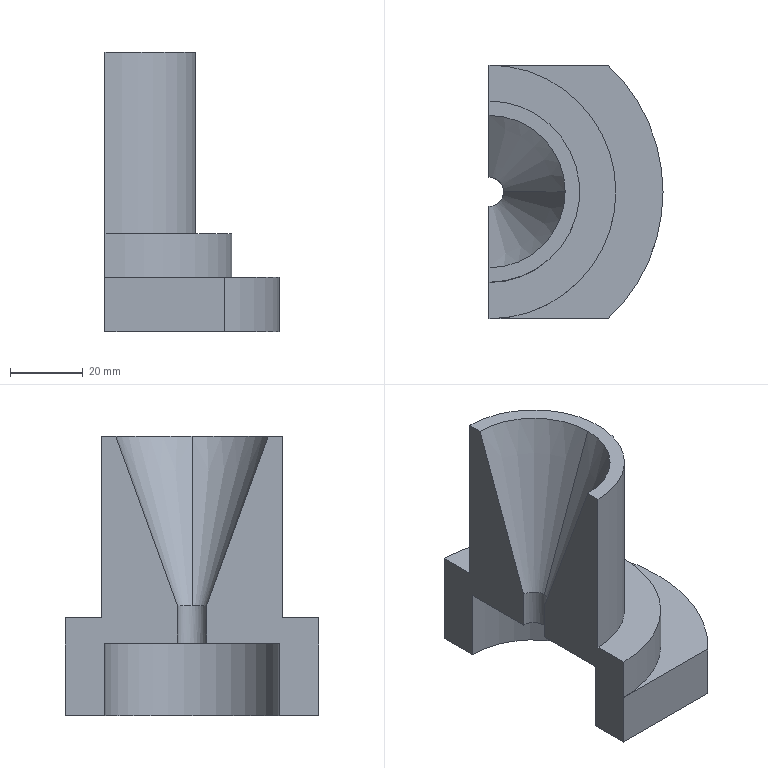Part | STEP file | 001-005-Shaft threading fixture mould | 1 solid | 16 faces | box 48 x 70 x 77 mm | volume 85963 mm3 | plane 9 | cylinder 5 | cone 2 | commonest cylinder face diameters 8.04 x1 48.1 x1 50 x1 70 x1 96 x1
STEP:
#1=CARTESIAN_POINT('',(0.,0.,0.));
#2=DIRECTION('',(0.,0.,1.));
#3=DIRECTION('',(1.,0.,0.));
#4=AXIS2_PLACEMENT_3D('',#1,#2,#3);
#5=CARTESIAN_POINT('',(0.,4.02,30.293));
#6=VERTEX_POINT('',#5);
#7=CARTESIAN_POINT('',(0.,21.02,77.));
#8=VERTEX_POINT('',#7);
#9=CARTESIAN_POINT('',(0.,0.,19.248));
#10=DIRECTION('',(0.,0.342,0.9397));
#11=VECTOR('',#10,1.);
#12=LINE('',#9,#11);
#13=CARTESIAN_POINT('',(0.,0.,77.));
#14=DIRECTION('',(0.,0.,1.));
#15=DIRECTION('',(1.,0.,0.));
#16=AXIS2_PLACEMENT_3D('',#13,#14,#15);
#17=CONICAL_SURFACE('',#16,21.02,0.3491);
#18=CARTESIAN_POINT('',(1.571,-57.752));
#19=DIRECTION('',(0.,1.));
#20=VECTOR('',#19,1.);
#21=LINE('',#18,#20);
#22=(GEOMETRIC_REPRESENTATION_CONTEXT(2)PARAMETRIC_REPRESENTATION_CONTEXT()REPRESENTATION_CONTEXT('',''));
#23=DEFINITIONAL_REPRESENTATION('',(#21),#22);
#24=PCURVE('',#17,#23);
#25=CARTESIAN_POINT('',(0.,0.,0.));
#26=DIRECTION('',(1.,0.,0.));
#27=DIRECTION('',(0.,0.,-1.));
#28=AXIS2_PLACEMENT_3D('',#25,#26,#27);
#29=PLANE('',#28);
#30=CARTESIAN_POINT('',(-19.248,0.));
#31=DIRECTION('',(-0.9397,0.342));
#32=VECTOR('',#31,1.);
#33=LINE('',#30,#32);
#34=(GEOMETRIC_REPRESENTATION_CONTEXT(2)PARAMETRIC_REPRESENTATION_CONTEXT()REPRESENTATION_CONTEXT('',''));
#35=DEFINITIONAL_REPRESENTATION('',(#33),#34);
#36=PCURVE('',#29,#35);
#37=SURFACE_CURVE('',#12,(#24,#36),.PCURVE_S1.);
#38=EDGE_CURVE('',#6,#8,#37,.T.);
#39=ORIENTED_EDGE('',*,*,#38,.T.);
#40=CARTESIAN_POINT('',(21.02,0.,77.));
#41=VERTEX_POINT('',#40);
#42=CARTESIAN_POINT('',(0.,0.,77.));
#43=DIRECTION('',(0.,0.,-1.));
#44=DIRECTION('',(1.,0.,0.));
#45=AXIS2_PLACEMENT_3D('',#42,#43,#44);
#46=CIRCLE('',#45,21.02);
#47=CARTESIAN_POINT('',(6.283,0.));
#48=DIRECTION('',(-1.,0.));
#49=VECTOR('',#48,1.);
#50=LINE('',#47,#49);
#51=(GEOMETRIC_REPRESENTATION_CONTEXT(2)PARAMETRIC_REPRESENTATION_CONTEXT()REPRESENTATION_CONTEXT('',''));
#52=DEFINITIONAL_REPRESENTATION('',(#50),#51);
#53=PCURVE('',#17,#52);
#54=CARTESIAN_POINT('',(0.,0.,77.));
#55=DIRECTION('',(0.,0.,1.));
#56=DIRECTION('',(1.,0.,0.));
#57=AXIS2_PLACEMENT_3D('',#54,#55,#56);
#58=PLANE('',#57);
#59=CARTESIAN_POINT('',(21.02,0.));
#60=CARTESIAN_POINT('',(21.02,-36.408));
#61=CARTESIAN_POINT('',(-10.51,-18.204));
#62=CARTESIAN_POINT('',(-42.04,0.));
#63=CARTESIAN_POINT('',(-10.51,18.204));
#64=CARTESIAN_POINT('',(21.02,36.408));
#65=CARTESIAN_POINT('',(21.02,0.));
#66=(BOUNDED_CURVE()B_SPLINE_CURVE(2,(#59,#60,#61,#62,#63,#64,#65),.UNSPECIFIED.,.T.,.F.)B_SPLINE_CURVE_WITH_KNOTS((1,2,2,2,2,1),(-2.094,0.,2.094,4.189,6.283,8.378),.UNSPECIFIED.)CURVE()GEOMETRIC_REPRESENTATION_ITEM()RATIONAL_B_SPLINE_CURVE((1.,0.5,1.,0.5,1.,0.5,1.))REPRESENTATION_ITEM(''));
#67=(GEOMETRIC_REPRESENTATION_CONTEXT(2)PARAMETRIC_REPRESENTATION_CONTEXT()REPRESENTATION_CONTEXT('',''));
#68=DEFINITIONAL_REPRESENTATION('',(#66),#67);
#69=PCURVE('',#58,#68);
#70=SURFACE_CURVE('',#46,(#53,#69),.PCURVE_S1.);
#71=EDGE_CURVE('',#8,#41,#70,.T.);
#72=ORIENTED_EDGE('',*,*,#71,.T.);
#73=CARTESIAN_POINT('',(4.02,0.,30.293));
#74=VERTEX_POINT('',#73);
#75=CARTESIAN_POINT('',(21.02,0.,77.));
#76=DIRECTION('',(0.342,0.,0.9397));
#77=VECTOR('',#76,1.);
#78=LINE('',#75,#77);
#79=CARTESIAN_POINT('',(0.,0.));
#80=DIRECTION('',(0.,1.));
#81=VECTOR('',#80,1.);
#82=LINE('',#79,#81);
#83=(GEOMETRIC_REPRESENTATION_CONTEXT(2)PARAMETRIC_REPRESENTATION_CONTEXT()REPRESENTATION_CONTEXT('',''));
#84=DEFINITIONAL_REPRESENTATION('',(#82),#83);
#85=PCURVE('',#17,#84);
#86=CARTESIAN_POINT('',(0.,0.,77.));
#87=DIRECTION('',(0.,0.,1.));
#88=DIRECTION('',(1.,0.,0.));
#89=AXIS2_PLACEMENT_3D('',#86,#87,#88);
#90=CONICAL_SURFACE('',#89,21.02,0.3491);
#91=CARTESIAN_POINT('',(6.283,0.));
#92=DIRECTION('',(0.,1.));
#93=VECTOR('',#92,1.);
#94=LINE('',#91,#93);
#95=(GEOMETRIC_REPRESENTATION_CONTEXT(2)PARAMETRIC_REPRESENTATION_CONTEXT()REPRESENTATION_CONTEXT('',''));
#96=DEFINITIONAL_REPRESENTATION('',(#94),#95);
#97=PCURVE('',#90,#96);
#98=SURFACE_CURVE('',#78,(#85,#97),.PCURVE_S1.);
#99=EDGE_CURVE('',#74,#41,#98,.T.);
#100=ORIENTED_EDGE('',*,*,#99,.F.);
#101=CARTESIAN_POINT('',(0.,0.,30.293));
#102=DIRECTION('',(0.,0.,1.));
#103=DIRECTION('',(1.,0.,0.));
#104=AXIS2_PLACEMENT_3D('',#101,#102,#103);
#105=CIRCLE('',#104,4.02);
#106=CARTESIAN_POINT('',(0.,-46.707));
#107=DIRECTION('',(1.,0.));
#108=VECTOR('',#107,1.);
#109=LINE('',#106,#108);
#110=(GEOMETRIC_REPRESENTATION_CONTEXT(2)PARAMETRIC_REPRESENTATION_CONTEXT()REPRESENTATION_CONTEXT('',''));
#111=DEFINITIONAL_REPRESENTATION('',(#109),#110);
#112=PCURVE('',#17,#111);
#113=CARTESIAN_POINT('',(0.,0.,77.));
#114=DIRECTION('',(0.,0.,-1.));
#115=DIRECTION('',(-1.,0.,0.));
#116=AXIS2_PLACEMENT_3D('',#113,#114,#115);
#117=CYLINDRICAL_SURFACE('',#116,4.02);
#118=CARTESIAN_POINT('',(3.142,46.707));
#119=DIRECTION('',(-1.,0.));
#120=VECTOR('',#119,1.);
#121=LINE('',#118,#120);
#122=(GEOMETRIC_REPRESENTATION_CONTEXT(2)PARAMETRIC_REPRESENTATION_CONTEXT()REPRESENTATION_CONTEXT('',''));
#123=DEFINITIONAL_REPRESENTATION('',(#121),#122);
#124=PCURVE('',#117,#123);
#125=SURFACE_CURVE('',#105,(#112,#124),.PCURVE_S1.);
#126=EDGE_CURVE('',#74,#6,#125,.T.);
#127=ORIENTED_EDGE('',*,*,#126,.T.);
#128=EDGE_LOOP('',(#39,#72,#100,#127));
#129=FACE_BOUND('',#128,.F.);
#130=ADVANCED_FACE('',(#129),#17,.F.);
#131=CARTESIAN_POINT('',(0.,-25.,77.));
#132=VERTEX_POINT('',#131);
#133=CARTESIAN_POINT('',(0.,-21.02,77.));
#134=VERTEX_POINT('',#133);
#135=CARTESIAN_POINT('',(0.,0.,77.));
#136=DIRECTION('',(0.,1.,0.));
#137=VECTOR('',#136,1.);
#138=LINE('',#135,#137);
#139=CARTESIAN_POINT('',(0.,0.,0.));
#140=DIRECTION('',(1.,0.,0.));
#141=DIRECTION('',(0.,0.,-1.));
#142=AXIS2_PLACEMENT_3D('',#139,#140,#141);
#143=PLANE('',#142);
#144=CARTESIAN_POINT('',(-77.,0.));
#145=DIRECTION('',(0.,1.));
#146=VECTOR('',#145,1.);
#147=LINE('',#144,#146);
#148=(GEOMETRIC_REPRESENTATION_CONTEXT(2)PARAMETRIC_REPRESENTATION_CONTEXT()REPRESENTATION_CONTEXT('',''));
#149=DEFINITIONAL_REPRESENTATION('',(#147),#148);
#150=PCURVE('',#143,#149);
#151=CARTESIAN_POINT('',(0.,0.));
#152=DIRECTION('',(0.,1.));
#153=VECTOR('',#152,1.);
#154=LINE('',#151,#153);
#155=(GEOMETRIC_REPRESENTATION_CONTEXT(2)PARAMETRIC_REPRESENTATION_CONTEXT()REPRESENTATION_CONTEXT('',''));
#156=DEFINITIONAL_REPRESENTATION('',(#154),#155);
#157=PCURVE('',#58,#156);
#158=SURFACE_CURVE('',#138,(#150,#157),.PCURVE_S1.);
#159=EDGE_CURVE('',#132,#134,#158,.T.);
#160=ORIENTED_EDGE('',*,*,#159,.T.);
#161=CARTESIAN_POINT('',(0.,-4.02,30.293));
#162=VERTEX_POINT('',#161);
#163=CARTESIAN_POINT('',(0.,0.,19.248));
#164=DIRECTION('',(0.,0.342,-0.9397));
#165=VECTOR('',#164,1.);
#166=LINE('',#163,#165);
#167=CARTESIAN_POINT('',(-19.248,0.));
#168=DIRECTION('',(0.9397,0.342));
#169=VECTOR('',#168,1.);
#170=LINE('',#167,#169);
#171=(GEOMETRIC_REPRESENTATION_CONTEXT(2)PARAMETRIC_REPRESENTATION_CONTEXT()REPRESENTATION_CONTEXT('',''));
#172=DEFINITIONAL_REPRESENTATION('',(#170),#171);
#173=PCURVE('',#143,#172);
#174=CARTESIAN_POINT('',(4.712,-57.752));
#175=DIRECTION('',(0.,-1.));
#176=VECTOR('',#175,1.);
#177=LINE('',#174,#176);
#178=(GEOMETRIC_REPRESENTATION_CONTEXT(2)PARAMETRIC_REPRESENTATION_CONTEXT()REPRESENTATION_CONTEXT('',''));
#179=DEFINITIONAL_REPRESENTATION('',(#177),#178);
#180=PCURVE('',#90,#179);
#181=SURFACE_CURVE('',#166,(#173,#180),.PCURVE_S1.);
#182=EDGE_CURVE('',#134,#162,#181,.T.);
#183=ORIENTED_EDGE('',*,*,#182,.T.);
#184=CARTESIAN_POINT('',(0.,-4.02,20.));
#185=VERTEX_POINT('',#184);
#186=CARTESIAN_POINT('',(0.,-4.02,77.));
#187=DIRECTION('',(0.,0.,1.));
#188=VECTOR('',#187,1.);
#189=LINE('',#186,#188);
#190=CARTESIAN_POINT('',(-77.,-4.02));
#191=DIRECTION('',(-1.,0.));
#192=VECTOR('',#191,1.);
#193=LINE('',#190,#192);
#194=(GEOMETRIC_REPRESENTATION_CONTEXT(2)PARAMETRIC_REPRESENTATION_CONTEXT()REPRESENTATION_CONTEXT('',''));
#195=DEFINITIONAL_REPRESENTATION('',(#193),#194);
#196=PCURVE('',#143,#195);
#197=CARTESIAN_POINT('',(4.712,0.));
#198=DIRECTION('',(0.,-1.));
#199=VECTOR('',#198,1.);
#200=LINE('',#197,#199);
#201=(GEOMETRIC_REPRESENTATION_CONTEXT(2)PARAMETRIC_REPRESENTATION_CONTEXT()REPRESENTATION_CONTEXT('',''));
#202=DEFINITIONAL_REPRESENTATION('',(#200),#201);
#203=PCURVE('',#117,#202);
#204=SURFACE_CURVE('',#189,(#196,#203),.PCURVE_S1.);
#205=EDGE_CURVE('',#185,#162,#204,.T.);
#206=ORIENTED_EDGE('',*,*,#205,.F.);
#207=CARTESIAN_POINT('',(0.,-24.05,20.));
#208=VERTEX_POINT('',#207);
#209=CARTESIAN_POINT('',(0.,0.,20.));
#210=DIRECTION('',(0.,-1.,0.));
#211=VECTOR('',#210,1.);
#212=LINE('',#209,#211);
#213=CARTESIAN_POINT('',(-20.,0.));
#214=DIRECTION('',(0.,-1.));
#215=VECTOR('',#214,1.);
#216=LINE('',#213,#215);
#217=(GEOMETRIC_REPRESENTATION_CONTEXT(2)PARAMETRIC_REPRESENTATION_CONTEXT()REPRESENTATION_CONTEXT('',''));
#218=DEFINITIONAL_REPRESENTATION('',(#216),#217);
#219=PCURVE('',#143,#218);
#220=CARTESIAN_POINT('',(0.,0.,20.));
#221=DIRECTION('',(0.,0.,-1.));
#222=DIRECTION('',(-1.,0.,0.));
#223=AXIS2_PLACEMENT_3D('',#220,#221,#222);
#224=PLANE('',#223);
#225=CARTESIAN_POINT('',(0.,0.));
#226=DIRECTION('',(0.,-1.));
#227=VECTOR('',#226,1.);
#228=LINE('',#225,#227);
#229=(GEOMETRIC_REPRESENTATION_CONTEXT(2)PARAMETRIC_REPRESENTATION_CONTEXT()REPRESENTATION_CONTEXT('',''));
#230=DEFINITIONAL_REPRESENTATION('',(#228),#229);
#231=PCURVE('',#224,#230);
#232=SURFACE_CURVE('',#212,(#219,#231),.PCURVE_S1.);
#233=EDGE_CURVE('',#185,#208,#232,.T.);
#234=ORIENTED_EDGE('',*,*,#233,.T.);
#235=CARTESIAN_POINT('',(0.,-24.05,0.));
#236=VERTEX_POINT('',#235);
#237=CARTESIAN_POINT('',(0.,-24.05,20.));
#238=DIRECTION('',(0.,0.,1.));
#239=VECTOR('',#238,1.);
#240=LINE('',#237,#239);
#241=CARTESIAN_POINT('',(-20.,-24.05));
#242=DIRECTION('',(-1.,0.));
#243=VECTOR('',#242,1.);
#244=LINE('',#241,#243);
#245=(GEOMETRIC_REPRESENTATION_CONTEXT(2)PARAMETRIC_REPRESENTATION_CONTEXT()REPRESENTATION_CONTEXT('',''));
#246=DEFINITIONAL_REPRESENTATION('',(#244),#245);
#247=PCURVE('',#143,#246);
#248=CARTESIAN_POINT('',(0.,0.,20.));
#249=DIRECTION('',(0.,0.,-1.));
#250=DIRECTION('',(-1.,0.,0.));
#251=AXIS2_PLACEMENT_3D('',#248,#249,#250);
#252=CYLINDRICAL_SURFACE('',#251,24.05);
#253=CARTESIAN_POINT('',(4.712,0.));
#254=DIRECTION('',(0.,-1.));
#255=VECTOR('',#254,1.);
#256=LINE('',#253,#255);
#257=(GEOMETRIC_REPRESENTATION_CONTEXT(2)PARAMETRIC_REPRESENTATION_CONTEXT()REPRESENTATION_CONTEXT('',''));
#258=DEFINITIONAL_REPRESENTATION('',(#256),#257);
#259=PCURVE('',#252,#258);
#260=SURFACE_CURVE('',#240,(#247,#259),.PCURVE_S1.);
#261=EDGE_CURVE('',#236,#208,#260,.T.);
#262=ORIENTED_EDGE('',*,*,#261,.F.);
#263=CARTESIAN_POINT('',(0.,-35.,0.));
#264=VERTEX_POINT('',#263);
#265=CARTESIAN_POINT('',(0.,0.,0.));
#266=DIRECTION('',(0.,1.,0.));
#267=VECTOR('',#266,1.);
#268=LINE('',#265,#267);
#269=CARTESIAN_POINT('',(0.,0.));
#270=DIRECTION('',(0.,1.));
#271=VECTOR('',#270,1.);
#272=LINE('',#269,#271);
#273=(GEOMETRIC_REPRESENTATION_CONTEXT(2)PARAMETRIC_REPRESENTATION_CONTEXT()REPRESENTATION_CONTEXT('',''));
#274=DEFINITIONAL_REPRESENTATION('',(#272),#273);
#275=PCURVE('',#143,#274);
#276=CARTESIAN_POINT('',(0.,0.,0.));
#277=DIRECTION('',(0.,0.,1.));
#278=DIRECTION('',(1.,0.,0.));
#279=AXIS2_PLACEMENT_3D('',#276,#277,#278);
#280=PLANE('',#279);
#281=CARTESIAN_POINT('',(0.,0.));
#282=DIRECTION('',(0.,1.));
#283=VECTOR('',#282,1.);
#284=LINE('',#281,#283);
#285=(GEOMETRIC_REPRESENTATION_CONTEXT(2)PARAMETRIC_REPRESENTATION_CONTEXT()REPRESENTATION_CONTEXT('',''));
#286=DEFINITIONAL_REPRESENTATION('',(#284),#285);
#287=PCURVE('',#280,#286);
#288=SURFACE_CURVE('',#268,(#275,#287),.PCURVE_S1.);
#289=EDGE_CURVE('',#264,#236,#288,.T.);
#290=ORIENTED_EDGE('',*,*,#289,.F.);
#291=CARTESIAN_POINT('',(0.,-35.,15.));
#292=VERTEX_POINT('',#291);
#293=CARTESIAN_POINT('',(0.,-35.,77.));
#294=DIRECTION('',(0.,0.,-1.));
#295=VECTOR('',#294,1.);
#296=LINE('',#293,#295);
#297=CARTESIAN_POINT('',(-77.,-35.));
#298=DIRECTION('',(1.,0.));
#299=VECTOR('',#298,1.);
#300=LINE('',#297,#299);
#301=(GEOMETRIC_REPRESENTATION_CONTEXT(2)PARAMETRIC_REPRESENTATION_CONTEXT()REPRESENTATION_CONTEXT('',''));
#302=DEFINITIONAL_REPRESENTATION('',(#300),#301);
#303=PCURVE('',#143,#302);
#304=CARTESIAN_POINT('',(-65.,-35.,77.));
#305=DIRECTION('',(0.,1.,0.));
#306=DIRECTION('',(-1.,0.,0.));
#307=AXIS2_PLACEMENT_3D('',#304,#305,#306);
#308=PLANE('',#307);
#309=CARTESIAN_POINT('',(-65.,0.));
#310=DIRECTION('',(0.,-1.));
#311=VECTOR('',#310,1.);
#312=LINE('',#309,#311);
#313=(GEOMETRIC_REPRESENTATION_CONTEXT(2)PARAMETRIC_REPRESENTATION_CONTEXT()REPRESENTATION_CONTEXT('',''));
#314=DEFINITIONAL_REPRESENTATION('',(#312),#313);
#315=PCURVE('',#308,#314);
#316=SURFACE_CURVE('',#296,(#303,#315),.PCURVE_S1.);
#317=EDGE_CURVE('',#292,#264,#316,.T.);
#318=ORIENTED_EDGE('',*,*,#317,.F.);
#319=CARTESIAN_POINT('',(0.,-35.,27.));
#320=VERTEX_POINT('',#319);
#321=CARTESIAN_POINT('',(0.,-35.,27.));
#322=DIRECTION('',(0.,0.,-1.));
#323=VECTOR('',#322,1.);
#324=LINE('',#321,#323);
#325=CARTESIAN_POINT('',(-27.,-35.));
#326=DIRECTION('',(1.,0.));
#327=VECTOR('',#326,1.);
#328=LINE('',#325,#327);
#329=(GEOMETRIC_REPRESENTATION_CONTEXT(2)PARAMETRIC_REPRESENTATION_CONTEXT()REPRESENTATION_CONTEXT('',''));
#330=DEFINITIONAL_REPRESENTATION('',(#328),#329);
#331=PCURVE('',#143,#330);
#332=CARTESIAN_POINT('',(0.,0.,27.));
#333=DIRECTION('',(0.,0.,-1.));
#334=DIRECTION('',(-1.,0.,0.));
#335=AXIS2_PLACEMENT_3D('',#332,#333,#334);
#336=CYLINDRICAL_SURFACE('',#335,35.);
#337=CARTESIAN_POINT('',(4.712,0.));
#338=DIRECTION('',(0.,1.));
#339=VECTOR('',#338,1.);
#340=LINE('',#337,#339);
#341=(GEOMETRIC_REPRESENTATION_CONTEXT(2)PARAMETRIC_REPRESENTATION_CONTEXT()REPRESENTATION_CONTEXT('',''));
#342=DEFINITIONAL_REPRESENTATION('',(#340),#341);
#343=PCURVE('',#336,#342);
#344=SURFACE_CURVE('',#324,(#331,#343),.PCURVE_S1.);
#345=EDGE_CURVE('',#320,#292,#344,.T.);
#346=ORIENTED_EDGE('',*,*,#345,.F.);
#347=CARTESIAN_POINT('',(0.,-25.,27.));
#348=VERTEX_POINT('',#347);
#349=CARTESIAN_POINT('',(0.,0.,27.));
#350=DIRECTION('',(0.,1.,0.));
#351=VECTOR('',#350,1.);
#352=LINE('',#349,#351);
#353=CARTESIAN_POINT('',(-27.,0.));
#354=DIRECTION('',(0.,1.));
#355=VECTOR('',#354,1.);
#356=LINE('',#353,#355);
#357=(GEOMETRIC_REPRESENTATION_CONTEXT(2)PARAMETRIC_REPRESENTATION_CONTEXT()REPRESENTATION_CONTEXT('',''));
#358=DEFINITIONAL_REPRESENTATION('',(#356),#357);
#359=PCURVE('',#143,#358);
#360=CARTESIAN_POINT('',(0.,0.,27.));
#361=DIRECTION('',(0.,0.,1.));
#362=DIRECTION('',(1.,0.,0.));
#363=AXIS2_PLACEMENT_3D('',#360,#361,#362);
#364=PLANE('',#363);
#365=CARTESIAN_POINT('',(0.,0.));
#366=DIRECTION('',(0.,1.));
#367=VECTOR('',#366,1.);
#368=LINE('',#365,#367);
#369=(GEOMETRIC_REPRESENTATION_CONTEXT(2)PARAMETRIC_REPRESENTATION_CONTEXT()REPRESENTATION_CONTEXT('',''));
#370=DEFINITIONAL_REPRESENTATION('',(#368),#369);
#371=PCURVE('',#364,#370);
#372=SURFACE_CURVE('',#352,(#359,#371),.PCURVE_S1.);
#373=EDGE_CURVE('',#320,#348,#372,.T.);
#374=ORIENTED_EDGE('',*,*,#373,.T.);
#375=CARTESIAN_POINT('',(0.,-25.,77.));
#376=DIRECTION('',(0.,0.,-1.));
#377=VECTOR('',#376,1.);
#378=LINE('',#375,#377);
#379=CARTESIAN_POINT('',(-77.,-25.));
#380=DIRECTION('',(1.,0.));
#381=VECTOR('',#380,1.);
#382=LINE('',#379,#381);
#383=(GEOMETRIC_REPRESENTATION_CONTEXT(2)PARAMETRIC_REPRESENTATION_CONTEXT()REPRESENTATION_CONTEXT('',''));
#384=DEFINITIONAL_REPRESENTATION('',(#382),#383);
#385=PCURVE('',#143,#384);
#386=CARTESIAN_POINT('',(0.,0.,77.));
#387=DIRECTION('',(0.,0.,-1.));
#388=DIRECTION('',(-1.,0.,0.));
#389=AXIS2_PLACEMENT_3D('',#386,#387,#388);
#390=CYLINDRICAL_SURFACE('',#389,25.);
#391=CARTESIAN_POINT('',(4.712,0.));
#392=DIRECTION('',(0.,1.));
#393=VECTOR('',#392,1.);
#394=LINE('',#391,#393);
#395=(GEOMETRIC_REPRESENTATION_CONTEXT(2)PARAMETRIC_REPRESENTATION_CONTEXT()REPRESENTATION_CONTEXT('',''));
#396=DEFINITIONAL_REPRESENTATION('',(#394),#395);
#397=PCURVE('',#390,#396);
#398=SURFACE_CURVE('',#378,(#385,#397),.PCURVE_S1.);
#399=EDGE_CURVE('',#132,#348,#398,.T.);
#400=ORIENTED_EDGE('',*,*,#399,.F.);
#401=EDGE_LOOP('',(#160,#183,#206,#234,#262,#290,#318,#346,#374,#400));
#402=FACE_BOUND('',#401,.T.);
#403=ADVANCED_FACE('',(#402),#143,.F.);
#404=CARTESIAN_POINT('',(32.848,-35.,0.));
#405=VERTEX_POINT('',#404);
#406=CARTESIAN_POINT('',(32.848,35.,0.));
#407=VERTEX_POINT('',#406);
#408=CARTESIAN_POINT('',(0.,0.,0.));
#409=DIRECTION('',(0.,0.,1.));
#410=DIRECTION('',(1.,0.,0.));
#411=AXIS2_PLACEMENT_3D('',#408,#409,#410);
#412=CIRCLE('',#411,48.);
#413=CARTESIAN_POINT('',(0.,0.,15.));
#414=DIRECTION('',(0.,0.,-1.));
#415=DIRECTION('',(-1.,0.,0.));
#416=AXIS2_PLACEMENT_3D('',#413,#414,#415);
#417=CYLINDRICAL_SURFACE('',#416,48.);
#418=CARTESIAN_POINT('',(9.425,15.));
#419=DIRECTION('',(-1.,0.));
#420=VECTOR('',#419,1.);
#421=LINE('',#418,#420);
#422=(GEOMETRIC_REPRESENTATION_CONTEXT(2)PARAMETRIC_REPRESENTATION_CONTEXT()REPRESENTATION_CONTEXT('',''));
#423=DEFINITIONAL_REPRESENTATION('',(#421),#422);
#424=PCURVE('',#417,#423);
#425=CARTESIAN_POINT('',(0.,0.));
#426=DIRECTION('',(1.,0.));
#427=AXIS2_PLACEMENT_2D('',#425,#426);
#428=CIRCLE('',#427,48.);
#429=(GEOMETRIC_REPRESENTATION_CONTEXT(2)PARAMETRIC_REPRESENTATION_CONTEXT()REPRESENTATION_CONTEXT('',''));
#430=DEFINITIONAL_REPRESENTATION('',(#428),#429);
#431=PCURVE('',#280,#430);
#432=SURFACE_CURVE('',#412,(#424,#431),.PCURVE_S1.);
#433=EDGE_CURVE('',#405,#407,#432,.T.);
#434=ORIENTED_EDGE('',*,*,#433,.T.);
#435=CARTESIAN_POINT('',(32.848,35.,15.));
#436=VERTEX_POINT('',#435);
#437=CARTESIAN_POINT('',(32.848,35.,15.));
#438=DIRECTION('',(0.,0.,1.));
#439=VECTOR('',#438,1.);
#440=LINE('',#437,#439);
#441=CARTESIAN_POINT('',(2.324,0.));
#442=DIRECTION('',(0.,-1.));
#443=VECTOR('',#442,1.);
#444=LINE('',#441,#443);
#445=(GEOMETRIC_REPRESENTATION_CONTEXT(2)PARAMETRIC_REPRESENTATION_CONTEXT()REPRESENTATION_CONTEXT('',''));
#446=DEFINITIONAL_REPRESENTATION('',(#444),#445);
#447=PCURVE('',#417,#446);
#448=CARTESIAN_POINT('',(-65.,35.,77.));
#449=DIRECTION('',(0.,-1.,0.));
#450=DIRECTION('',(0.,0.,-1.));
#451=AXIS2_PLACEMENT_3D('',#448,#449,#450);
#452=PLANE('',#451);
#453=CARTESIAN_POINT('',(62.,97.848));
#454=DIRECTION('',(-1.,0.));
#455=VECTOR('',#454,1.);
#456=LINE('',#453,#455);
#457=(GEOMETRIC_REPRESENTATION_CONTEXT(2)PARAMETRIC_REPRESENTATION_CONTEXT()REPRESENTATION_CONTEXT('',''));
#458=DEFINITIONAL_REPRESENTATION('',(#456),#457);
#459=PCURVE('',#452,#458);
#460=SURFACE_CURVE('',#440,(#447,#459),.PCURVE_S1.);
#461=EDGE_CURVE('',#407,#436,#460,.T.);
#462=ORIENTED_EDGE('',*,*,#461,.T.);
#463=CARTESIAN_POINT('',(32.848,-35.,15.));
#464=VERTEX_POINT('',#463);
#465=CARTESIAN_POINT('',(0.,0.,15.));
#466=DIRECTION('',(0.,0.,1.));
#467=DIRECTION('',(1.,0.,0.));
#468=AXIS2_PLACEMENT_3D('',#465,#466,#467);
#469=CIRCLE('',#468,48.);
#470=CARTESIAN_POINT('',(9.425,0.));
#471=DIRECTION('',(-1.,0.));
#472=VECTOR('',#471,1.);
#473=LINE('',#470,#472);
#474=(GEOMETRIC_REPRESENTATION_CONTEXT(2)PARAMETRIC_REPRESENTATION_CONTEXT()REPRESENTATION_CONTEXT('',''));
#475=DEFINITIONAL_REPRESENTATION('',(#473),#474);
#476=PCURVE('',#417,#475);
#477=CARTESIAN_POINT('',(0.,0.,15.));
#478=DIRECTION('',(0.,0.,1.));
#479=DIRECTION('',(1.,0.,0.));
#480=AXIS2_PLACEMENT_3D('',#477,#478,#479);
#481=PLANE('',#480);
#482=CARTESIAN_POINT('',(0.,0.));
#483=DIRECTION('',(1.,0.));
#484=AXIS2_PLACEMENT_2D('',#482,#483);
#485=CIRCLE('',#484,48.);
#486=(GEOMETRIC_REPRESENTATION_CONTEXT(2)PARAMETRIC_REPRESENTATION_CONTEXT()REPRESENTATION_CONTEXT('',''));
#487=DEFINITIONAL_REPRESENTATION('',(#485),#486);
#488=PCURVE('',#481,#487);
#489=SURFACE_CURVE('',#469,(#476,#488),.PCURVE_S1.);
#490=EDGE_CURVE('',#464,#436,#489,.T.);
#491=ORIENTED_EDGE('',*,*,#490,.F.);
#492=CARTESIAN_POINT('',(32.848,-35.,15.));
#493=DIRECTION('',(0.,0.,-1.));
#494=VECTOR('',#493,1.);
#495=LINE('',#492,#494);
#496=CARTESIAN_POINT('',(3.959,0.));
#497=DIRECTION('',(0.,1.));
#498=VECTOR('',#497,1.);
#499=LINE('',#496,#498);
#500=(GEOMETRIC_REPRESENTATION_CONTEXT(2)PARAMETRIC_REPRESENTATION_CONTEXT()REPRESENTATION_CONTEXT('',''));
#501=DEFINITIONAL_REPRESENTATION('',(#499),#500);
#502=PCURVE('',#417,#501);
#503=CARTESIAN_POINT('',(-97.848,-62.));
#504=DIRECTION('',(0.,-1.));
#505=VECTOR('',#504,1.);
#506=LINE('',#503,#505);
#507=(GEOMETRIC_REPRESENTATION_CONTEXT(2)PARAMETRIC_REPRESENTATION_CONTEXT()REPRESENTATION_CONTEXT('',''));
#508=DEFINITIONAL_REPRESENTATION('',(#506),#507);
#509=PCURVE('',#308,#508);
#510=SURFACE_CURVE('',#495,(#502,#509),.PCURVE_S1.);
#511=EDGE_CURVE('',#464,#405,#510,.T.);
#512=ORIENTED_EDGE('',*,*,#511,.T.);
#513=EDGE_LOOP('',(#434,#462,#491,#512));
#514=FACE_BOUND('',#513,.T.);
#515=ADVANCED_FACE('',(#514),#417,.T.);
#516=CARTESIAN_POINT('',(0.,35.,15.));
#517=VERTEX_POINT('',#516);
#518=CARTESIAN_POINT('',(0.,35.,15.));
#519=DIRECTION('',(1.,0.,0.));
#520=VECTOR('',#519,1.);
#521=LINE('',#518,#520);
#522=CARTESIAN_POINT('',(0.,35.));
#523=DIRECTION('',(1.,0.));
#524=VECTOR('',#523,1.);
#525=LINE('',#522,#524);
#526=(GEOMETRIC_REPRESENTATION_CONTEXT(2)PARAMETRIC_REPRESENTATION_CONTEXT()REPRESENTATION_CONTEXT('',''));
#527=DEFINITIONAL_REPRESENTATION('',(#525),#526);
#528=PCURVE('',#481,#527);
#529=CARTESIAN_POINT('',(62.,65.));
#530=DIRECTION('',(0.,1.));
#531=VECTOR('',#530,1.);
#532=LINE('',#529,#531);
#533=(GEOMETRIC_REPRESENTATION_CONTEXT(2)PARAMETRIC_REPRESENTATION_CONTEXT()REPRESENTATION_CONTEXT('',''));
#534=DEFINITIONAL_REPRESENTATION('',(#532),#533);
#535=PCURVE('',#452,#534);
#536=SURFACE_CURVE('',#521,(#528,#535),.PCURVE_S1.);
#537=EDGE_CURVE('',#517,#436,#536,.T.);
#538=ORIENTED_EDGE('',*,*,#537,.F.);
#539=CARTESIAN_POINT('',(0.,0.,15.));
#540=DIRECTION('',(0.,0.,1.));
#541=DIRECTION('',(1.,0.,0.));
#542=AXIS2_PLACEMENT_3D('',#539,#540,#541);
#543=CIRCLE('',#542,35.);
#544=CARTESIAN_POINT('',(0.,0.));
#545=DIRECTION('',(1.,0.));
#546=AXIS2_PLACEMENT_2D('',#544,#545);
#547=CIRCLE('',#546,35.);
#548=(GEOMETRIC_REPRESENTATION_CONTEXT(2)PARAMETRIC_REPRESENTATION_CONTEXT()REPRESENTATION_CONTEXT('',''));
#549=DEFINITIONAL_REPRESENTATION('',(#547),#548);
#550=PCURVE('',#481,#549);
#551=CARTESIAN_POINT('',(9.425,12.));
#552=DIRECTION('',(-1.,0.));
#553=VECTOR('',#552,1.);
#554=LINE('',#551,#553);
#555=(GEOMETRIC_REPRESENTATION_CONTEXT(2)PARAMETRIC_REPRESENTATION_CONTEXT()REPRESENTATION_CONTEXT('',''));
#556=DEFINITIONAL_REPRESENTATION('',(#554),#555);
#557=PCURVE('',#336,#556);
#558=SURFACE_CURVE('',#543,(#550,#557),.PCURVE_S1.);
#559=EDGE_CURVE('',#292,#517,#558,.T.);
#560=ORIENTED_EDGE('',*,*,#559,.F.);
#561=CARTESIAN_POINT('',(0.,-35.,15.));
#562=DIRECTION('',(-1.,0.,0.));
#563=VECTOR('',#562,1.);
#564=LINE('',#561,#563);
#565=CARTESIAN_POINT('',(0.,-35.));
#566=DIRECTION('',(-1.,0.));
#567=VECTOR('',#566,1.);
#568=LINE('',#565,#567);
#569=(GEOMETRIC_REPRESENTATION_CONTEXT(2)PARAMETRIC_REPRESENTATION_CONTEXT()REPRESENTATION_CONTEXT('',''));
#570=DEFINITIONAL_REPRESENTATION('',(#568),#569);
#571=PCURVE('',#481,#570);
#572=CARTESIAN_POINT('',(-65.,-62.));
#573=DIRECTION('',(1.,0.));
#574=VECTOR('',#573,1.);
#575=LINE('',#572,#574);
#576=(GEOMETRIC_REPRESENTATION_CONTEXT(2)PARAMETRIC_REPRESENTATION_CONTEXT()REPRESENTATION_CONTEXT('',''));
#577=DEFINITIONAL_REPRESENTATION('',(#575),#576);
#578=PCURVE('',#308,#577);
#579=SURFACE_CURVE('',#564,(#571,#578),.PCURVE_S1.);
#580=EDGE_CURVE('',#464,#292,#579,.T.);
#581=ORIENTED_EDGE('',*,*,#580,.F.);
#582=ORIENTED_EDGE('',*,*,#490,.T.);
#583=EDGE_LOOP('',(#538,#560,#581,#582));
#584=FACE_BOUND('',#583,.T.);
#585=ADVANCED_FACE('',(#584),#481,.T.);
#586=CARTESIAN_POINT('',(-65.,-35.,0.));
#587=DIRECTION('',(1.,0.,0.));
#588=VECTOR('',#587,1.);
#589=LINE('',#586,#588);
#590=CARTESIAN_POINT('',(-65.,-35.));
#591=DIRECTION('',(1.,0.));
#592=VECTOR('',#591,1.);
#593=LINE('',#590,#592);
#594=(GEOMETRIC_REPRESENTATION_CONTEXT(2)PARAMETRIC_REPRESENTATION_CONTEXT()REPRESENTATION_CONTEXT('',''));
#595=DEFINITIONAL_REPRESENTATION('',(#593),#594);
#596=PCURVE('',#280,#595);
#597=CARTESIAN_POINT('',(0.,-77.));
#598=DIRECTION('',(-1.,0.));
#599=VECTOR('',#598,1.);
#600=LINE('',#597,#599);
#601=(GEOMETRIC_REPRESENTATION_CONTEXT(2)PARAMETRIC_REPRESENTATION_CONTEXT()REPRESENTATION_CONTEXT('',''));
#602=DEFINITIONAL_REPRESENTATION('',(#600),#601);
#603=PCURVE('',#308,#602);
#604=SURFACE_CURVE('',#589,(#596,#603),.PCURVE_S1.);
#605=EDGE_CURVE('',#264,#405,#604,.T.);
#606=ORIENTED_EDGE('',*,*,#605,.F.);
#607=ORIENTED_EDGE('',*,*,#289,.T.);
#608=CARTESIAN_POINT('',(0.,24.05,0.));
#609=VERTEX_POINT('',#608);
#610=CARTESIAN_POINT('',(0.,0.,0.));
#611=DIRECTION('',(0.,0.,-1.));
#612=DIRECTION('',(-1.,0.,0.));
#613=AXIS2_PLACEMENT_3D('',#610,#611,#612);
#614=CIRCLE('',#613,24.05);
#615=CARTESIAN_POINT('',(-24.05,0.));
#616=CARTESIAN_POINT('',(-24.05,41.656));
#617=CARTESIAN_POINT('',(12.025,20.828));
#618=CARTESIAN_POINT('',(48.1,0.));
#619=CARTESIAN_POINT('',(12.025,-20.828));
#620=CARTESIAN_POINT('',(-24.05,-41.656));
#621=CARTESIAN_POINT('',(-24.05,0.));
#622=(BOUNDED_CURVE()B_SPLINE_CURVE(2,(#615,#616,#617,#618,#619,#620,#621),.UNSPECIFIED.,.T.,.F.)B_SPLINE_CURVE_WITH_KNOTS((1,2,2,2,2,1),(-2.094,0.,2.094,4.189,6.283,8.378),.UNSPECIFIED.)CURVE()GEOMETRIC_REPRESENTATION_ITEM()RATIONAL_B_SPLINE_CURVE((1.,0.5,1.,0.5,1.,0.5,1.))REPRESENTATION_ITEM(''));
#623=(GEOMETRIC_REPRESENTATION_CONTEXT(2)PARAMETRIC_REPRESENTATION_CONTEXT()REPRESENTATION_CONTEXT('',''));
#624=DEFINITIONAL_REPRESENTATION('',(#622),#623);
#625=PCURVE('',#280,#624);
#626=CARTESIAN_POINT('',(0.,20.));
#627=DIRECTION('',(1.,0.));
#628=VECTOR('',#627,1.);
#629=LINE('',#626,#628);
#630=(GEOMETRIC_REPRESENTATION_CONTEXT(2)PARAMETRIC_REPRESENTATION_CONTEXT()REPRESENTATION_CONTEXT('',''));
#631=DEFINITIONAL_REPRESENTATION('',(#629),#630);
#632=PCURVE('',#252,#631);
#633=SURFACE_CURVE('',#614,(#625,#632),.PCURVE_S1.);
#634=EDGE_CURVE('',#609,#236,#633,.T.);
#635=ORIENTED_EDGE('',*,*,#634,.F.);
#636=CARTESIAN_POINT('',(0.,35.,0.));
#637=VERTEX_POINT('',#636);
#638=CARTESIAN_POINT('',(0.,0.,0.));
#639=DIRECTION('',(0.,1.,0.));
#640=VECTOR('',#639,1.);
#641=LINE('',#638,#640);
#642=CARTESIAN_POINT('',(0.,0.));
#643=DIRECTION('',(0.,1.));
#644=VECTOR('',#643,1.);
#645=LINE('',#642,#644);
#646=(GEOMETRIC_REPRESENTATION_CONTEXT(2)PARAMETRIC_REPRESENTATION_CONTEXT()REPRESENTATION_CONTEXT('',''));
#647=DEFINITIONAL_REPRESENTATION('',(#645),#646);
#648=PCURVE('',#280,#647);
#649=CARTESIAN_POINT('',(0.,0.));
#650=DIRECTION('',(0.,1.));
#651=VECTOR('',#650,1.);
#652=LINE('',#649,#651);
#653=(GEOMETRIC_REPRESENTATION_CONTEXT(2)PARAMETRIC_REPRESENTATION_CONTEXT()REPRESENTATION_CONTEXT('',''));
#654=DEFINITIONAL_REPRESENTATION('',(#652),#653);
#655=PCURVE('',#29,#654);
#656=SURFACE_CURVE('',#641,(#648,#655),.PCURVE_S1.);
#657=EDGE_CURVE('',#609,#637,#656,.T.);
#658=ORIENTED_EDGE('',*,*,#657,.T.);
#659=CARTESIAN_POINT('',(-65.,35.,0.));
#660=DIRECTION('',(-1.,0.,0.));
#661=VECTOR('',#660,1.);
#662=LINE('',#659,#661);
#663=CARTESIAN_POINT('',(-65.,35.));
#664=DIRECTION('',(-1.,0.));
#665=VECTOR('',#664,1.);
#666=LINE('',#663,#665);
#667=(GEOMETRIC_REPRESENTATION_CONTEXT(2)PARAMETRIC_REPRESENTATION_CONTEXT()REPRESENTATION_CONTEXT('',''));
#668=DEFINITIONAL_REPRESENTATION('',(#666),#667);
#669=PCURVE('',#280,#668);
#670=CARTESIAN_POINT('',(77.,0.));
#671=DIRECTION('',(0.,-1.));
#672=VECTOR('',#671,1.);
#673=LINE('',#670,#672);
#674=(GEOMETRIC_REPRESENTATION_CONTEXT(2)PARAMETRIC_REPRESENTATION_CONTEXT()REPRESENTATION_CONTEXT('',''));
#675=DEFINITIONAL_REPRESENTATION('',(#673),#674);
#676=PCURVE('',#452,#675);
#677=SURFACE_CURVE('',#662,(#669,#676),.PCURVE_S1.);
#678=EDGE_CURVE('',#407,#637,#677,.T.);
#679=ORIENTED_EDGE('',*,*,#678,.F.);
#680=ORIENTED_EDGE('',*,*,#433,.F.);
#681=EDGE_LOOP('',(#606,#607,#635,#658,#679,#680));
#682=FACE_BOUND('',#681,.T.);
#683=ADVANCED_FACE('',(#682),#280,.F.);
#684=CARTESIAN_POINT('',(0.,35.,27.));
#685=VERTEX_POINT('',#684);
#686=CARTESIAN_POINT('',(0.,0.,27.));
#687=DIRECTION('',(0.,0.,1.));
#688=DIRECTION('',(1.,0.,0.));
#689=AXIS2_PLACEMENT_3D('',#686,#687,#688);
#690=CIRCLE('',#689,35.);
#691=CARTESIAN_POINT('',(9.425,0.));
#692=DIRECTION('',(-1.,0.));
#693=VECTOR('',#692,1.);
#694=LINE('',#691,#693);
#695=(GEOMETRIC_REPRESENTATION_CONTEXT(2)PARAMETRIC_REPRESENTATION_CONTEXT()REPRESENTATION_CONTEXT('',''));
#696=DEFINITIONAL_REPRESENTATION('',(#694),#695);
#697=PCURVE('',#336,#696);
#698=CARTESIAN_POINT('',(0.,0.));
#699=DIRECTION('',(1.,0.));
#700=AXIS2_PLACEMENT_2D('',#698,#699);
#701=CIRCLE('',#700,35.);
#702=(GEOMETRIC_REPRESENTATION_CONTEXT(2)PARAMETRIC_REPRESENTATION_CONTEXT()REPRESENTATION_CONTEXT('',''));
#703=DEFINITIONAL_REPRESENTATION('',(#701),#702);
#704=PCURVE('',#364,#703);
#705=SURFACE_CURVE('',#690,(#697,#704),.PCURVE_S1.);
#706=EDGE_CURVE('',#320,#685,#705,.T.);
#707=ORIENTED_EDGE('',*,*,#706,.F.);
#708=ORIENTED_EDGE('',*,*,#345,.T.);
#709=ORIENTED_EDGE('',*,*,#559,.T.);
#710=CARTESIAN_POINT('',(0.,35.,27.));
#711=DIRECTION('',(0.,0.,1.));
#712=VECTOR('',#711,1.);
#713=LINE('',#710,#712);
#714=CARTESIAN_POINT('',(1.571,0.));
#715=DIRECTION('',(0.,-1.));
#716=VECTOR('',#715,1.);
#717=LINE('',#714,#716);
#718=(GEOMETRIC_REPRESENTATION_CONTEXT(2)PARAMETRIC_REPRESENTATION_CONTEXT()REPRESENTATION_CONTEXT('',''));
#719=DEFINITIONAL_REPRESENTATION('',(#717),#718);
#720=PCURVE('',#336,#719);
#721=CARTESIAN_POINT('',(-27.,35.));
#722=DIRECTION('',(-1.,0.));
#723=VECTOR('',#722,1.);
#724=LINE('',#721,#723);
#725=(GEOMETRIC_REPRESENTATION_CONTEXT(2)PARAMETRIC_REPRESENTATION_CONTEXT()REPRESENTATION_CONTEXT('',''));
#726=DEFINITIONAL_REPRESENTATION('',(#724),#725);
#727=PCURVE('',#29,#726);
#728=SURFACE_CURVE('',#713,(#720,#727),.PCURVE_S1.);
#729=EDGE_CURVE('',#517,#685,#728,.T.);
#730=ORIENTED_EDGE('',*,*,#729,.T.);
#731=EDGE_LOOP('',(#707,#708,#709,#730));
#732=FACE_BOUND('',#731,.T.);
#733=ADVANCED_FACE('',(#732),#336,.T.);
#734=ORIENTED_EDGE('',*,*,#373,.F.);
#735=ORIENTED_EDGE('',*,*,#706,.T.);
#736=CARTESIAN_POINT('',(0.,25.,27.));
#737=VERTEX_POINT('',#736);
#738=CARTESIAN_POINT('',(0.,0.,27.));
#739=DIRECTION('',(0.,1.,0.));
#740=VECTOR('',#739,1.);
#741=LINE('',#738,#740);
#742=CARTESIAN_POINT('',(0.,0.));
#743=DIRECTION('',(0.,1.));
#744=VECTOR('',#743,1.);
#745=LINE('',#742,#744);
#746=(GEOMETRIC_REPRESENTATION_CONTEXT(2)PARAMETRIC_REPRESENTATION_CONTEXT()REPRESENTATION_CONTEXT('',''));
#747=DEFINITIONAL_REPRESENTATION('',(#745),#746);
#748=PCURVE('',#364,#747);
#749=CARTESIAN_POINT('',(-27.,0.));
#750=DIRECTION('',(0.,1.));
#751=VECTOR('',#750,1.);
#752=LINE('',#749,#751);
#753=(GEOMETRIC_REPRESENTATION_CONTEXT(2)PARAMETRIC_REPRESENTATION_CONTEXT()REPRESENTATION_CONTEXT('',''));
#754=DEFINITIONAL_REPRESENTATION('',(#752),#753);
#755=PCURVE('',#29,#754);
#756=SURFACE_CURVE('',#741,(#748,#755),.PCURVE_S1.);
#757=EDGE_CURVE('',#737,#685,#756,.T.);
#758=ORIENTED_EDGE('',*,*,#757,.F.);
#759=CARTESIAN_POINT('',(0.,0.,27.));
#760=DIRECTION('',(0.,0.,1.));
#761=DIRECTION('',(1.,0.,0.));
#762=AXIS2_PLACEMENT_3D('',#759,#760,#761);
#763=CIRCLE('',#762,25.);
#764=CARTESIAN_POINT('',(0.,0.));
#765=DIRECTION('',(1.,0.));
#766=AXIS2_PLACEMENT_2D('',#764,#765);
#767=CIRCLE('',#766,25.);
#768=(GEOMETRIC_REPRESENTATION_CONTEXT(2)PARAMETRIC_REPRESENTATION_CONTEXT()REPRESENTATION_CONTEXT('',''));
#769=DEFINITIONAL_REPRESENTATION('',(#767),#768);
#770=PCURVE('',#364,#769);
#771=CARTESIAN_POINT('',(9.425,50.));
#772=DIRECTION('',(-1.,0.));
#773=VECTOR('',#772,1.);
#774=LINE('',#771,#773);
#775=(GEOMETRIC_REPRESENTATION_CONTEXT(2)PARAMETRIC_REPRESENTATION_CONTEXT()REPRESENTATION_CONTEXT('',''));
#776=DEFINITIONAL_REPRESENTATION('',(#774),#775);
#777=PCURVE('',#390,#776);
#778=SURFACE_CURVE('',#763,(#770,#777),.PCURVE_S1.);
#779=EDGE_CURVE('',#348,#737,#778,.T.);
#780=ORIENTED_EDGE('',*,*,#779,.F.);
#781=EDGE_LOOP('',(#734,#735,#758,#780));
#782=FACE_BOUND('',#781,.T.);
#783=ADVANCED_FACE('',(#782),#364,.T.);
#784=CARTESIAN_POINT('',(0.,25.,77.));
#785=VERTEX_POINT('',#784);
#786=CARTESIAN_POINT('',(0.,0.,77.));
#787=DIRECTION('',(0.,0.,1.));
#788=DIRECTION('',(1.,0.,0.));
#789=AXIS2_PLACEMENT_3D('',#786,#787,#788);
#790=CIRCLE('',#789,25.);
#791=CARTESIAN_POINT('',(9.425,0.));
#792=DIRECTION('',(-1.,0.));
#793=VECTOR('',#792,1.);
#794=LINE('',#791,#793);
#795=(GEOMETRIC_REPRESENTATION_CONTEXT(2)PARAMETRIC_REPRESENTATION_CONTEXT()REPRESENTATION_CONTEXT('',''));
#796=DEFINITIONAL_REPRESENTATION('',(#794),#795);
#797=PCURVE('',#390,#796);
#798=CARTESIAN_POINT('',(0.,0.));
#799=DIRECTION('',(1.,0.));
#800=AXIS2_PLACEMENT_2D('',#798,#799);
#801=CIRCLE('',#800,25.);
#802=(GEOMETRIC_REPRESENTATION_CONTEXT(2)PARAMETRIC_REPRESENTATION_CONTEXT()REPRESENTATION_CONTEXT('',''));
#803=DEFINITIONAL_REPRESENTATION('',(#801),#802);
#804=PCURVE('',#58,#803);
#805=SURFACE_CURVE('',#790,(#797,#804),.PCURVE_S1.);
#806=EDGE_CURVE('',#132,#785,#805,.T.);
#807=ORIENTED_EDGE('',*,*,#806,.F.);
#808=ORIENTED_EDGE('',*,*,#399,.T.);
#809=ORIENTED_EDGE('',*,*,#779,.T.);
#810=CARTESIAN_POINT('',(0.,25.,77.));
#811=DIRECTION('',(0.,0.,1.));
#812=VECTOR('',#811,1.);
#813=LINE('',#810,#812);
#814=CARTESIAN_POINT('',(1.571,0.));
#815=DIRECTION('',(0.,-1.));
#816=VECTOR('',#815,1.);
#817=LINE('',#814,#816);
#818=(GEOMETRIC_REPRESENTATION_CONTEXT(2)PARAMETRIC_REPRESENTATION_CONTEXT()REPRESENTATION_CONTEXT('',''));
#819=DEFINITIONAL_REPRESENTATION('',(#817),#818);
#820=PCURVE('',#390,#819);
#821=CARTESIAN_POINT('',(-77.,25.));
#822=DIRECTION('',(-1.,0.));
#823=VECTOR('',#822,1.);
#824=LINE('',#821,#823);
#825=(GEOMETRIC_REPRESENTATION_CONTEXT(2)PARAMETRIC_REPRESENTATION_CONTEXT()REPRESENTATION_CONTEXT('',''));
#826=DEFINITIONAL_REPRESENTATION('',(#824),#825);
#827=PCURVE('',#29,#826);
#828=SURFACE_CURVE('',#813,(#820,#827),.PCURVE_S1.);
#829=EDGE_CURVE('',#737,#785,#828,.T.);
#830=ORIENTED_EDGE('',*,*,#829,.T.);
#831=EDGE_LOOP('',(#807,#808,#809,#830));
#832=FACE_BOUND('',#831,.T.);
#833=ADVANCED_FACE('',(#832),#390,.T.);
#834=ORIENTED_EDGE('',*,*,#159,.F.);
#835=ORIENTED_EDGE('',*,*,#806,.T.);
#836=CARTESIAN_POINT('',(0.,0.,77.));
#837=DIRECTION('',(0.,1.,0.));
#838=VECTOR('',#837,1.);
#839=LINE('',#836,#838);
#840=CARTESIAN_POINT('',(0.,0.));
#841=DIRECTION('',(0.,1.));
#842=VECTOR('',#841,1.);
#843=LINE('',#840,#842);
#844=(GEOMETRIC_REPRESENTATION_CONTEXT(2)PARAMETRIC_REPRESENTATION_CONTEXT()REPRESENTATION_CONTEXT('',''));
#845=DEFINITIONAL_REPRESENTATION('',(#843),#844);
#846=PCURVE('',#58,#845);
#847=CARTESIAN_POINT('',(-77.,0.));
#848=DIRECTION('',(0.,1.));
#849=VECTOR('',#848,1.);
#850=LINE('',#847,#849);
#851=(GEOMETRIC_REPRESENTATION_CONTEXT(2)PARAMETRIC_REPRESENTATION_CONTEXT()REPRESENTATION_CONTEXT('',''));
#852=DEFINITIONAL_REPRESENTATION('',(#850),#851);
#853=PCURVE('',#29,#852);
#854=SURFACE_CURVE('',#839,(#846,#853),.PCURVE_S1.);
#855=EDGE_CURVE('',#8,#785,#854,.T.);
#856=ORIENTED_EDGE('',*,*,#855,.F.);
#857=ORIENTED_EDGE('',*,*,#71,.T.);
#858=CARTESIAN_POINT('',(0.,0.,77.));
#859=DIRECTION('',(0.,0.,-1.));
#860=DIRECTION('',(1.,0.,0.));
#861=AXIS2_PLACEMENT_3D('',#858,#859,#860);
#862=CIRCLE('',#861,21.02);
#863=CARTESIAN_POINT('',(21.02,0.));
#864=CARTESIAN_POINT('',(21.02,-36.408));
#865=CARTESIAN_POINT('',(-10.51,-18.204));
#866=CARTESIAN_POINT('',(-42.04,0.));
#867=CARTESIAN_POINT('',(-10.51,18.204));
#868=CARTESIAN_POINT('',(21.02,36.408));
#869=CARTESIAN_POINT('',(21.02,0.));
#870=(BOUNDED_CURVE()B_SPLINE_CURVE(2,(#863,#864,#865,#866,#867,#868,#869),.UNSPECIFIED.,.T.,.F.)B_SPLINE_CURVE_WITH_KNOTS((1,2,2,2,2,1),(-2.094,0.,2.094,4.189,6.283,8.378),.UNSPECIFIED.)CURVE()GEOMETRIC_REPRESENTATION_ITEM()RATIONAL_B_SPLINE_CURVE((1.,0.5,1.,0.5,1.,0.5,1.))REPRESENTATION_ITEM(''));
#871=(GEOMETRIC_REPRESENTATION_CONTEXT(2)PARAMETRIC_REPRESENTATION_CONTEXT()REPRESENTATION_CONTEXT('',''));
#872=DEFINITIONAL_REPRESENTATION('',(#870),#871);
#873=PCURVE('',#58,#872);
#874=CARTESIAN_POINT('',(6.283,0.));
#875=DIRECTION('',(-1.,0.));
#876=VECTOR('',#875,1.);
#877=LINE('',#874,#876);
#878=(GEOMETRIC_REPRESENTATION_CONTEXT(2)PARAMETRIC_REPRESENTATION_CONTEXT()REPRESENTATION_CONTEXT('',''));
#879=DEFINITIONAL_REPRESENTATION('',(#877),#878);
#880=PCURVE('',#90,#879);
#881=SURFACE_CURVE('',#862,(#873,#880),.PCURVE_S1.);
#882=EDGE_CURVE('',#41,#134,#881,.T.);
#883=ORIENTED_EDGE('',*,*,#882,.T.);
#884=EDGE_LOOP('',(#834,#835,#856,#857,#883));
#885=FACE_BOUND('',#884,.T.);
#886=ADVANCED_FACE('',(#885),#58,.T.);
#887=CARTESIAN_POINT('',(0.,24.05,20.));
#888=VERTEX_POINT('',#887);
#889=CARTESIAN_POINT('',(0.,24.05,20.));
#890=DIRECTION('',(0.,0.,-1.));
#891=VECTOR('',#890,1.);
#892=LINE('',#889,#891);
#893=CARTESIAN_POINT('',(1.571,0.));
#894=DIRECTION('',(0.,1.));
#895=VECTOR('',#894,1.);
#896=LINE('',#893,#895);
#897=(GEOMETRIC_REPRESENTATION_CONTEXT(2)PARAMETRIC_REPRESENTATION_CONTEXT()REPRESENTATION_CONTEXT('',''));
#898=DEFINITIONAL_REPRESENTATION('',(#896),#897);
#899=PCURVE('',#252,#898);
#900=CARTESIAN_POINT('',(-20.,24.05));
#901=DIRECTION('',(1.,0.));
#902=VECTOR('',#901,1.);
#903=LINE('',#900,#902);
#904=(GEOMETRIC_REPRESENTATION_CONTEXT(2)PARAMETRIC_REPRESENTATION_CONTEXT()REPRESENTATION_CONTEXT('',''));
#905=DEFINITIONAL_REPRESENTATION('',(#903),#904);
#906=PCURVE('',#29,#905);
#907=SURFACE_CURVE('',#892,(#899,#906),.PCURVE_S1.);
#908=EDGE_CURVE('',#888,#609,#907,.T.);
#909=ORIENTED_EDGE('',*,*,#908,.F.);
#910=CARTESIAN_POINT('',(0.,0.,20.));
#911=DIRECTION('',(0.,0.,-1.));
#912=DIRECTION('',(-1.,0.,0.));
#913=AXIS2_PLACEMENT_3D('',#910,#911,#912);
#914=CIRCLE('',#913,24.05);
#915=CARTESIAN_POINT('',(0.,0.));
#916=DIRECTION('',(1.,0.));
#917=VECTOR('',#916,1.);
#918=LINE('',#915,#917);
#919=(GEOMETRIC_REPRESENTATION_CONTEXT(2)PARAMETRIC_REPRESENTATION_CONTEXT()REPRESENTATION_CONTEXT('',''));
#920=DEFINITIONAL_REPRESENTATION('',(#918),#919);
#921=PCURVE('',#252,#920);
#922=CARTESIAN_POINT('',(0.,0.));
#923=DIRECTION('',(1.,0.));
#924=AXIS2_PLACEMENT_2D('',#922,#923);
#925=CIRCLE('',#924,24.05);
#926=(GEOMETRIC_REPRESENTATION_CONTEXT(2)PARAMETRIC_REPRESENTATION_CONTEXT()REPRESENTATION_CONTEXT('',''));
#927=DEFINITIONAL_REPRESENTATION('',(#925),#926);
#928=PCURVE('',#224,#927);
#929=SURFACE_CURVE('',#914,(#921,#928),.PCURVE_S1.);
#930=EDGE_CURVE('',#888,#208,#929,.T.);
#931=ORIENTED_EDGE('',*,*,#930,.T.);
#932=ORIENTED_EDGE('',*,*,#261,.F.);
#933=ORIENTED_EDGE('',*,*,#634,.F.);
#934=EDGE_LOOP('',(#909,#931,#932,#933));
#935=FACE_BOUND('',#934,.F.);
#936=ADVANCED_FACE('',(#935),#252,.F.);
#937=CARTESIAN_POINT('',(0.,4.02,20.));
#938=VERTEX_POINT('',#937);
#939=CARTESIAN_POINT('',(0.,0.,20.));
#940=DIRECTION('',(0.,-1.,0.));
#941=VECTOR('',#940,1.);
#942=LINE('',#939,#941);
#943=CARTESIAN_POINT('',(0.,0.));
#944=DIRECTION('',(0.,-1.));
#945=VECTOR('',#944,1.);
#946=LINE('',#943,#945);
#947=(GEOMETRIC_REPRESENTATION_CONTEXT(2)PARAMETRIC_REPRESENTATION_CONTEXT()REPRESENTATION_CONTEXT('',''));
#948=DEFINITIONAL_REPRESENTATION('',(#946),#947);
#949=PCURVE('',#224,#948);
#950=CARTESIAN_POINT('',(-20.,0.));
#951=DIRECTION('',(0.,-1.));
#952=VECTOR('',#951,1.);
#953=LINE('',#950,#952);
#954=(GEOMETRIC_REPRESENTATION_CONTEXT(2)PARAMETRIC_REPRESENTATION_CONTEXT()REPRESENTATION_CONTEXT('',''));
#955=DEFINITIONAL_REPRESENTATION('',(#953),#954);
#956=PCURVE('',#29,#955);
#957=SURFACE_CURVE('',#942,(#949,#956),.PCURVE_S1.);
#958=EDGE_CURVE('',#888,#938,#957,.T.);
#959=ORIENTED_EDGE('',*,*,#958,.F.);
#960=ORIENTED_EDGE('',*,*,#930,.T.);
#961=ORIENTED_EDGE('',*,*,#233,.F.);
#962=CARTESIAN_POINT('',(0.,0.,20.));
#963=DIRECTION('',(0.,0.,-1.));
#964=DIRECTION('',(-1.,0.,0.));
#965=AXIS2_PLACEMENT_3D('',#962,#963,#964);
#966=CIRCLE('',#965,4.02);
#967=CARTESIAN_POINT('',(0.,0.));
#968=DIRECTION('',(1.,0.));
#969=AXIS2_PLACEMENT_2D('',#967,#968);
#970=CIRCLE('',#969,4.02);
#971=(GEOMETRIC_REPRESENTATION_CONTEXT(2)PARAMETRIC_REPRESENTATION_CONTEXT()REPRESENTATION_CONTEXT('',''));
#972=DEFINITIONAL_REPRESENTATION('',(#970),#971);
#973=PCURVE('',#224,#972);
#974=CARTESIAN_POINT('',(0.,57.));
#975=DIRECTION('',(1.,0.));
#976=VECTOR('',#975,1.);
#977=LINE('',#974,#976);
#978=(GEOMETRIC_REPRESENTATION_CONTEXT(2)PARAMETRIC_REPRESENTATION_CONTEXT()REPRESENTATION_CONTEXT('',''));
#979=DEFINITIONAL_REPRESENTATION('',(#977),#978);
#980=PCURVE('',#117,#979);
#981=SURFACE_CURVE('',#966,(#973,#980),.PCURVE_S1.);
#982=EDGE_CURVE('',#938,#185,#981,.T.);
#983=ORIENTED_EDGE('',*,*,#982,.F.);
#984=EDGE_LOOP('',(#959,#960,#961,#983));
#985=FACE_BOUND('',#984,.T.);
#986=ADVANCED_FACE('',(#985),#224,.T.);
#987=CARTESIAN_POINT('',(0.,4.02,77.));
#988=DIRECTION('',(0.,0.,-1.));
#989=VECTOR('',#988,1.);
#990=LINE('',#987,#989);
#991=CARTESIAN_POINT('',(1.571,0.));
#992=DIRECTION('',(0.,1.));
#993=VECTOR('',#992,1.);
#994=LINE('',#991,#993);
#995=(GEOMETRIC_REPRESENTATION_CONTEXT(2)PARAMETRIC_REPRESENTATION_CONTEXT()REPRESENTATION_CONTEXT('',''));
#996=DEFINITIONAL_REPRESENTATION('',(#994),#995);
#997=PCURVE('',#117,#996);
#998=CARTESIAN_POINT('',(-77.,4.02));
#999=DIRECTION('',(1.,0.));
#1000=VECTOR('',#999,1.);
#1001=LINE('',#998,#1000);
#1002=(GEOMETRIC_REPRESENTATION_CONTEXT(2)PARAMETRIC_REPRESENTATION_CONTEXT()REPRESENTATION_CONTEXT('',''));
#1003=DEFINITIONAL_REPRESENTATION('',(#1001),#1002);
#1004=PCURVE('',#29,#1003);
#1005=SURFACE_CURVE('',#990,(#997,#1004),.PCURVE_S1.);
#1006=EDGE_CURVE('',#6,#938,#1005,.T.);
#1007=ORIENTED_EDGE('',*,*,#1006,.F.);
#1008=ORIENTED_EDGE('',*,*,#126,.F.);
#1009=CARTESIAN_POINT('',(0.,0.,30.293));
#1010=DIRECTION('',(0.,0.,1.));
#1011=DIRECTION('',(1.,0.,0.));
#1012=AXIS2_PLACEMENT_3D('',#1009,#1010,#1011);
#1013=CIRCLE('',#1012,4.02);
#1014=CARTESIAN_POINT('',(9.425,46.707));
#1015=DIRECTION('',(-1.,0.));
#1016=VECTOR('',#1015,1.);
#1017=LINE('',#1014,#1016);
#1018=(GEOMETRIC_REPRESENTATION_CONTEXT(2)PARAMETRIC_REPRESENTATION_CONTEXT()REPRESENTATION_CONTEXT('',''));
#1019=DEFINITIONAL_REPRESENTATION('',(#1017),#1018);
#1020=PCURVE('',#117,#1019);
#1021=CARTESIAN_POINT('',(0.,-46.707));
#1022=DIRECTION('',(1.,0.));
#1023=VECTOR('',#1022,1.);
#1024=LINE('',#1021,#1023);
#1025=(GEOMETRIC_REPRESENTATION_CONTEXT(2)PARAMETRIC_REPRESENTATION_CONTEXT()REPRESENTATION_CONTEXT('',''));
#1026=DEFINITIONAL_REPRESENTATION('',(#1024),#1025);
#1027=PCURVE('',#90,#1026);
#1028=SURFACE_CURVE('',#1013,(#1020,#1027),.PCURVE_S1.);
#1029=EDGE_CURVE('',#162,#74,#1028,.T.);
#1030=ORIENTED_EDGE('',*,*,#1029,.F.);
#1031=ORIENTED_EDGE('',*,*,#205,.F.);
#1032=ORIENTED_EDGE('',*,*,#982,.F.);
#1033=EDGE_LOOP('',(#1007,#1008,#1030,#1031,#1032));
#1034=FACE_BOUND('',#1033,.F.);
#1035=ADVANCED_FACE('',(#1034),#117,.F.);
#1036=ORIENTED_EDGE('',*,*,#882,.T.);
#1037=ORIENTED_EDGE('',*,*,#182,.T.);
#1038=ORIENTED_EDGE('',*,*,#1029,.T.);
#1039=ORIENTED_EDGE('',*,*,#99,.T.);
#1040=EDGE_LOOP('',(#1036,#1037,#1038,#1039));
#1041=FACE_BOUND('',#1040,.F.);
#1042=ADVANCED_FACE('',(#1041),#90,.F.);
#1043=ORIENTED_EDGE('',*,*,#580,.T.);
#1044=ORIENTED_EDGE('',*,*,#317,.T.);
#1045=ORIENTED_EDGE('',*,*,#605,.T.);
#1046=ORIENTED_EDGE('',*,*,#511,.F.);
#1047=EDGE_LOOP('',(#1043,#1044,#1045,#1046));
#1048=FACE_BOUND('',#1047,.T.);
#1049=ADVANCED_FACE('',(#1048),#308,.F.);
#1050=ORIENTED_EDGE('',*,*,#678,.T.);
#1051=CARTESIAN_POINT('',(0.,35.,77.));
#1052=DIRECTION('',(0.,0.,1.));
#1053=VECTOR('',#1052,1.);
#1054=LINE('',#1051,#1053);
#1055=CARTESIAN_POINT('',(0.,65.));
#1056=DIRECTION('',(-1.,0.));
#1057=VECTOR('',#1056,1.);
#1058=LINE('',#1055,#1057);
#1059=(GEOMETRIC_REPRESENTATION_CONTEXT(2)PARAMETRIC_REPRESENTATION_CONTEXT()REPRESENTATION_CONTEXT('',''));
#1060=DEFINITIONAL_REPRESENTATION('',(#1058),#1059);
#1061=PCURVE('',#452,#1060);
#1062=CARTESIAN_POINT('',(-77.,35.));
#1063=DIRECTION('',(-1.,0.));
#1064=VECTOR('',#1063,1.);
#1065=LINE('',#1062,#1064);
#1066=(GEOMETRIC_REPRESENTATION_CONTEXT(2)PARAMETRIC_REPRESENTATION_CONTEXT()REPRESENTATION_CONTEXT('',''));
#1067=DEFINITIONAL_REPRESENTATION('',(#1065),#1066);
#1068=PCURVE('',#29,#1067);
#1069=SURFACE_CURVE('',#1054,(#1061,#1068),.PCURVE_S1.);
#1070=EDGE_CURVE('',#637,#517,#1069,.T.);
#1071=ORIENTED_EDGE('',*,*,#1070,.T.);
#1072=ORIENTED_EDGE('',*,*,#537,.T.);
#1073=ORIENTED_EDGE('',*,*,#461,.F.);
#1074=EDGE_LOOP('',(#1050,#1071,#1072,#1073));
#1075=FACE_BOUND('',#1074,.T.);
#1076=ADVANCED_FACE('',(#1075),#452,.F.);
#1077=ORIENTED_EDGE('',*,*,#1006,.F.);
#1078=ORIENTED_EDGE('',*,*,#38,.T.);
#1079=ORIENTED_EDGE('',*,*,#855,.T.);
#1080=ORIENTED_EDGE('',*,*,#829,.F.);
#1081=ORIENTED_EDGE('',*,*,#757,.T.);
#1082=ORIENTED_EDGE('',*,*,#729,.F.);
#1083=ORIENTED_EDGE('',*,*,#1070,.F.);
#1084=ORIENTED_EDGE('',*,*,#657,.F.);
#1085=ORIENTED_EDGE('',*,*,#908,.F.);
#1086=ORIENTED_EDGE('',*,*,#958,.T.);
#1087=EDGE_LOOP('',(#1077,#1078,#1079,#1080,#1081,#1082,#1083,#1084,#1085,#1086));
#1088=FACE_BOUND('',#1087,.T.);
#1089=ADVANCED_FACE('',(#1088),#29,.F.);
#1090=CLOSED_SHELL('',(#130,#403,#515,#585,#683,#733,#783,#833,#886,#936,#986,#1035,#1042,#1049,#1076,#1089));
#1091=MANIFOLD_SOLID_BREP('',#1090);
#1092=(LENGTH_UNIT()NAMED_UNIT(*)SI_UNIT(.MILLI.,.METRE.));
#1093=UNCERTAINTY_MEASURE_WITH_UNIT(LENGTH_MEASURE(0.0000001),#1092,'','');
#1094=(NAMED_UNIT(*)PLANE_ANGLE_UNIT()SI_UNIT($,.RADIAN.));
#1095=(NAMED_UNIT(*)SI_UNIT($,.STERADIAN.)SOLID_ANGLE_UNIT());
#1096=(GEOMETRIC_REPRESENTATION_CONTEXT(3)GLOBAL_UNCERTAINTY_ASSIGNED_CONTEXT((#1093))GLOBAL_UNIT_ASSIGNED_CONTEXT((#1092,#1094,#1095))REPRESENTATION_CONTEXT('',''));
#1097=ADVANCED_BREP_SHAPE_REPRESENTATION('',(#4,#1091),#1096);